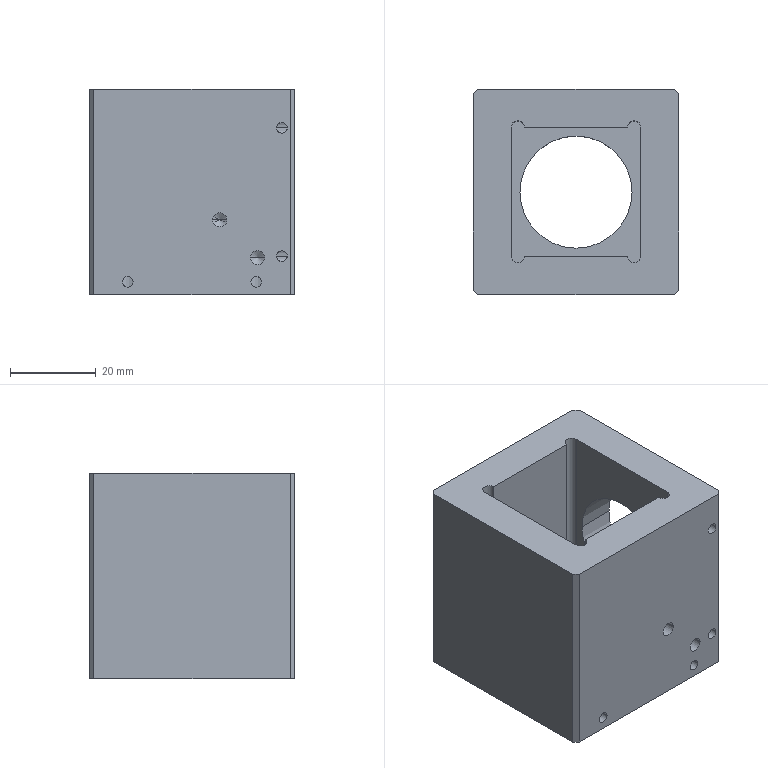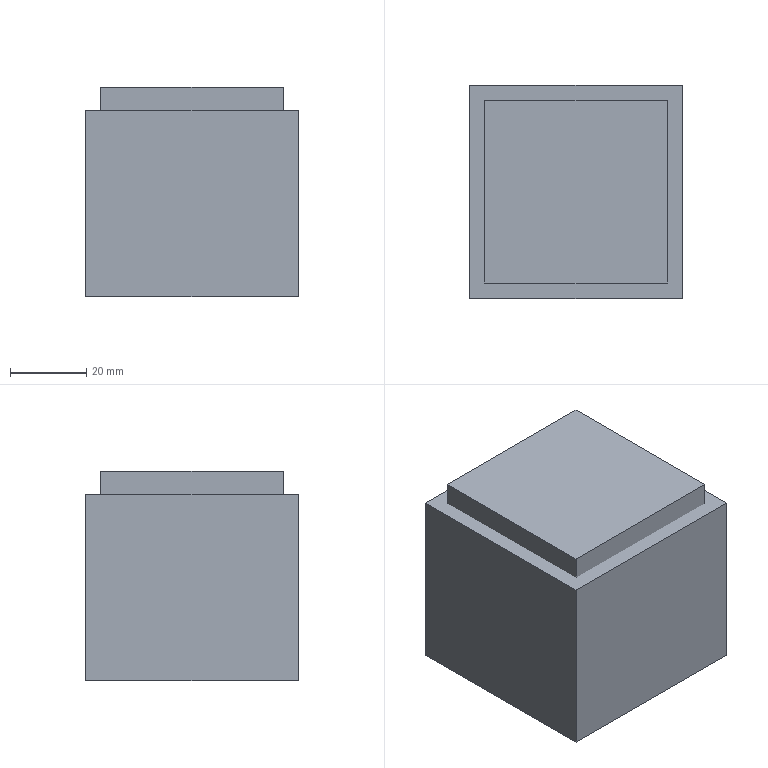CAM job | NX | 3+2 milling, drilling | part box 48 x 48 x 48 mm | stock box 56 x 56 x 55 mm
Tools:
number,name,description,diameter,corner_radius,flute_length,length,flutes
19,D80,Milling Tool-5 Parameters,80.0,0.0,50.0,75.0,2
1,D6A45,Milling Tool-5 Parameters,6.0,0.0,50.0,75.0,2
3,3.3ZT,Drilling Tool,3.3,0.0,35.0,50.0,2
16,3.0ZT,Drilling Tool,3.0,0.0,35.0,50.0,2
15,D10,Milling Tool-5 Parameters,10.0,0.0,50.0,75.0,2
14,D10JING,Milling Tool-5 Parameters,10.0,0.0,50.0,75.0,2
12,D6,Milling Tool-5 Parameters,6.0,0.0,50.0,75.0,2
11,D4,Milling Tool-5 Parameters,4.0,0.0,50.0,75.0,2
2,2.5ZT,Drilling Tool,2.5,0.0,35.0,50.0,2
Operations:
program,operation,operation_type,tool,method,geometry_group,spindle_rpm,surface_speed,feed_per_tooth,feed_cut,feed_plunge,cut_length_mm,path_length_mm,cut_time_min,machine_time_min
1,FLOOR_WALL_COPY,VolumeBased25DMillingOperation,D80,METHOD,A,6500.0,1633.0,0.1154,1500.0,100.0,152.0,206.0,0.1013,0.1067
1,DRILLING_COPY_1,Operation,D6A45,METHOD,A,5000.0,94.0,0.035,350.0,0.0,16.0,186.078,0.0457,0.0627
1,DRILLING_COPY_1_COPY_1_1_COPY_1,Operation,3.0ZT,METHOD,A,2000.0,18.0,0.025,100.0,0.0,171.605,513.662,1.716,1.75
1,ZLEVEL_PROFILE,ZLevelMilling,D10,METHOD,A,9500.0,298.0,0.1684,3200.0,1000.0,10748.532,10853.532,3.392,3.402
1,FLOOR_WALL,VolumeBased25DMillingOperation,D10,METHOD,A,9500.0,298.0,0.1316,2500.0,1000.0,7184.553,7627.862,4.107,4.152
1,ZLEVEL_PROFILE_1,ZLevelMilling,D6,METHOD,A,9500.0,179.0,0.0526,1000.0,100.0,2292.49,3563.367,2.292,2.42
1,ZLEVEL_PROFILE_1_COPY,ZLevelMilling,D4,METHOD,A,8000.0,100.0,0.05,800.0,100.0,2548.522,3812.041,3.186,3.312
1,FLOOR_WALL_COPY_1,VolumeBased25DMillingOperation,D10JING,METHOD,A,9500.0,298.0,0.0579,1100.0,1000.0,184.268,318.268,0.1723,0.1857
1,ZLEVEL_PROFILE_COPY_1_COPY_COPY_1_COPY_COPY,ZLevelMilling,D10JING,METHOD,A,9500.0,298.0,0.0632,1200.0,1000.0,685.234,1057.953,0.5728,0.6101
1,PLANAR_MILL_COPY_COPY_COPY_COPY_COPY_COPY_1_COPY_1,PlanarMilling,D6A45,METHOD,A,9500.0,179.0,0.0658,1250.0,100.0,327.495,456.995,0.262,0.2749
1,刀补12,ZLevelMilling,D6,METHOD,A,8000.0,150.0,0.0563,900.0,1000.0,718.048,1438.118,0.7954,0.8674
2,FLOOR_WALL_COPY_COPY,VolumeBased25DMillingOperation,D80,METHOD,B,6500.0,1633.0,0.1154,1500.0,100.0,1008.0,2172.002,0.672,0.7884
2,HOLE_MILLING,CylinderMilling,D10,METHOD,B,9500.0,298.0,0.1168,2220.0,100.0,829.664,907.664,0.3737,0.3815
2,ZLEVEL_PROFILE_COPY_1_COPY_COPY_1_COPY_COPY_COPY,ZLevelMilling,D10JING,METHOD,B,9500.0,298.0,0.0632,1200.0,1000.0,60.299,136.299,0.0511,0.0587
2,HOLE_MILLING_1,CylinderMilling,D4,METHOD,B,9500.0,119.0,0.0868,1650.0,100.0,374.069,724.069,0.2267,0.2617
2,PLANAR_MILL_COPY_COPY_COPY_COPY_COPY_COPY_1_COPY_1_COPY,PlanarMilling,D6A45,METHOD,B,9500.0,179.0,0.0658,1250.0,100.0,357.825,825.072,0.2863,0.333
2,刀补11,CylinderMilling,D4,METHOD,B,9500.0,119.0,0.0526,1000.0,100.0,111.438,461.438,0.1114,0.1464
3,HOLE_MILLING_COPY,CylinderMilling,D10,METHOD,C,9500.0,298.0,0.1168,2220.0,100.0,822.121,899.921,0.3703,0.3781
3,ZLEVEL_PROFILE_COPY_1_COPY_COPY_1_COPY_COPY_COPY_COPY,ZLevelMilling,D10JING,METHOD,C,9500.0,298.0,0.0632,1200.0,1000.0,59.16,134.96,0.05,0.0576
3,HOLE_MILLING_1_COPY,CylinderMilling,D4,METHOD,C,9500.0,119.0,0.0868,1650.0,100.0,391.076,742.276,0.237,0.2721
3,PLANAR_MILL_COPY_COPY_COPY_COPY_COPY_COPY_1_COPY_1_COPY_COPY,PlanarMilling,D6A45,METHOD,C,9500.0,179.0,0.0658,1250.0,100.0,167.107,551.178,0.1337,0.1721
3,刀补11_COPY,CylinderMilling,D4,METHOD,C,9500.0,119.0,0.0526,1000.0,100.0,115.216,466.416,0.1152,0.1503
4,DRILLING_COPY_1_COPY,Operation,D6A45,METHOD,D,5000.0,94.0,0.035,350.0,0.0,28.0,219.793,0.08,0.0992
4,DRILLING_COPY_1_COPY_1_1_COPY_1_COPY,Operation,2.5ZT,METHOD,D,2000.0,15.0,0.02,80.0,0.0,211.004,560.308,2.638,2.672
4,DRILLING_COPY_1_COPY_1_1_COPY_1_1,Operation,3.3ZT,METHOD,D,2000.0,34.0,0.05,200.0,0.0,29.974,151.658,0.1499,0.162
4,PLANAR_MILL_COPY_COPY_COPY_COPY_COPY_COPY_1_COPY_1_COPY_COPY_COPY,PlanarMilling,D6A45,METHOD,D,9500.0,179.0,0.0658,1250.0,100.0,81.019,576.156,0.0648,0.1143
5,DRILLING_COPY_1_COPY_COPY,Operation,D6A45,METHOD,E,5000.0,94.0,0.035,350.0,0.0,24.0,207.526,0.0686,0.0869
5,DRILLING_COPY_1_COPY_1_1_COPY_1_1_COPY,Operation,3.3ZT,METHOD,E,2000.0,34.0,0.05,200.0,0.0,19.983,115.821,0.0999,0.1095
5,PLANAR_MILL_COPY_COPY_COPY_COPY_COPY_COPY_1_COPY_1_COPY_COPY_COPY_COPY,PlanarMilling,D6A45,METHOD,E,9500.0,179.0,0.0658,1250.0,100.0,67.859,503.695,0.0543,0.0979